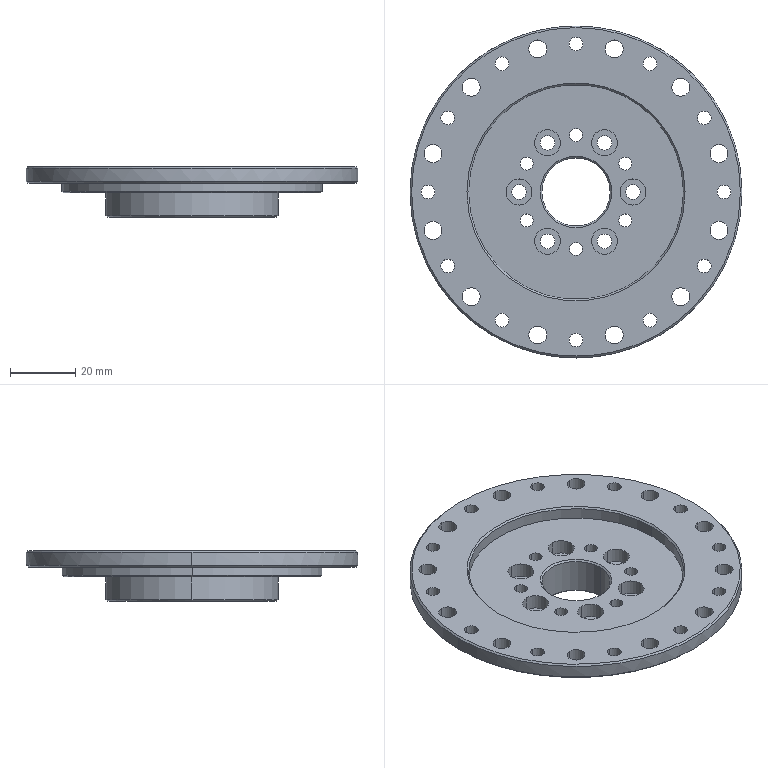NC program | NX | posted with a generic post | part box 102 x 102 x 15.5 mm
Whole program:
N10 G17 G21 G94 G90
(FLOOR_WALL_COPY_COPY , TOOL : D80)
N12 T19 M6
N14 G54
N16 G17 G0 G90 X-81.531 Y50.698 S6500 M3
N18 G43 Z30. H19
N20 Z12.
N22 G94 G1 Z9. F1500.
N24 X-75.579
N26 X75.578
N28 G2 X77.47 Y47.754 R90.667
N30 X89.618 Y15.852 R90.478
N32 G1 X-89.612
N34 G3 X-88.992 Y-18.994 R90.516
N36 G1 X89.006
N38 X94.112
N40 Z12.
N42 G0 Z30.
N44 X-81.542 Y50.698
N46 Z11.
N48 G1 Z8.
N50 X-75.59
N52 X75.572
N54 X75.681 Y50.534
N56 G2 X76.632 Y49.084 R90.524
N58 X89.618 Y15.851 R90.478
N60 G1 X-89.612
N62 G3 X-88.992 Y-18.995 R90.518
N64 G1 X89.006
N66 X94.112
N68 Z11.
N70 G0 Z30.
N72 X-81.541 Y50.699
N74 Z10.
N76 G1 Z7.
N78 X-75.589
N80 X75.571
N82 X75.653 Y50.576
N84 G2 X76.743 Y48.911 R90.596
N86 X89.618 Y15.852 R90.524
N88 G1 X-89.612
N90 G3 X-89.007 Y-18.995 R90.812
N92 G1 X89.006
N94 X94.112
N96 Z10.
N98 G0 Z30.
N100 X-81.535 Y50.701
N102 Z9.
N104 G1 Z6.
N106 X-75.582
N108 X75.576
N110 G2 X78.482 Y46.074 R90.403
N112 X88.337 Y21.908 R90.596
N114 X89.622 Y15.853 R90.962
N116 G1 X-89.622
N118 G3 X-90.747 Y6.882 R90.768
N120 X-90.99 Y1.917 R90.747
N122 G1 Y-1.978
N124 G3 X-90.558 Y-9.09 R90.747
N126 X-89.008 Y-18.995 R90.681
N128 G1 X89.009
N130 X94.116
N132 Z9.
N134 G0 Z30.
N136 X-81.535 Y50.698
N138 Z8.
N140 G1 Z5.
N142 X-75.581
N144 X75.578
N146 G2 X79.118 Y44.973 R90.403
N148 X86.435 Y28.496 R90.915
N150 X89.622 Y15.851 R90.962
N152 G1 X-89.622
N154 G3 X-90.737 Y7.019 R90.768
N156 X-90.939 Y3.54 R91.005
N158 X-90.99 Y1.854 R90.681
N160 G1 Y-1.943
N162 G3 X-89.008 Y-18.995 R90.681
N164 G1 X89.009
N166 X94.116
N168 Z8.
N170 G0 Z30.
N172 X-81.531 Y50.698
N174 Z7.
N176 G1 Z4.
N178 X-75.579
N180 X75.58
N182 G2 X88.039 Y23.072 R90.662
N184 X89.621 Y15.851 R90.915
N186 G1 X-89.617
N188 G3 X-90.99 Y1.81 R91.006
N190 G1 Y-1.809
N192 G3 X-89.003 Y-18.995 R91.006
N194 G1 X89.013
N196 X94.119
N198 Z7.
N200 G0 Z30.
N202 X-81.536 Y50.698
N204 Z6.
N206 G1 Z3.
N208 X-75.58
N210 X75.58
N212 G2 X89.013 Y18.957 R90.662
N214 X89.24 Y17.856 R90.754
N216 X89.618 Y15.851 R90.976
N218 G1 X-89.627
N220 G3 X-90.987 Y1.939 R89.934
N222 G1 X-90.99 Y1.81
N224 Y-1.83
N226 G3 X-89.005 Y-18.996 R90.93
N228 G1 X89.013
N230 X94.119
N232 Z6.
N234 G0 Z30.
N236 X-81.538 Y50.698
N238 Z5.
N240 G1 Z2.
N242 X-75.584
N244 X75.579
N246 G2 X86.561 Y28.116 R90.754
N248 X89.621 Y15.851 R90.903
N250 G1 X-89.627
N252 G3 X-90.99 Y1.827 R89.934
N254 G1 Y-1.83
N256 G3 X-89.005 Y-18.996 R90.93
N258 G1 X89.006
N260 X94.112
N262 Z5.
N264 G0 Z30.
N266 X-81.538 Y50.698
N268 Z4.
N270 G1 Z1.
N272 X-75.584
N274 X75.578
N276 G2 X89.621 Y15.851 R90.903
N278 G1 X-89.627
N280 G3 X-90.737 Y7.102 R89.96
N282 X-90.99 Y2.113 R90.464
N284 G1 Y-2.053
N286 G3 X-90.158 Y-12.385 R90.464
N288 X-89.004 Y-18.996 R90.725
N290 G1 X89.006
N292 X94.112
N294 Z4.
N296 G0 Z30.
N298 X-81.531 Y50.698
N300 Z3.
N302 G1 Z0.
N304 X-75.579
N306 X75.578
N308 G2 X80.872 Y41.745 R90.903
N310 X86.703 Y27.673 R90.662
N312 X89.621 Y15.852 R90.903
N314 G1 X-89.62
N316 G3 X-90.99 Y2.113 R90.464
N318 G1 Y-2.053
N320 G3 X-90.158 Y-12.385 R90.464
N322 G1 X-89.877 Y-14.187
N324 X-89.58 Y-16.052
N326 X-88.992 Y-18.994
N328 X89.006
N330 X94.112
N332 Z3.
N334 G0 Z30.
N336 M5
(ADAPTIVE_MILLING_COPY , TOOL : D10)
N338 T15 M6
N340 G54
N342 G17 G0 G90 X-62.764 Y0.058 S9500 M3
N344 G43 Z30. H15
N346 Z-7.35
N348 G94 G1 Z-10.35 F1000.
N350 X-60.098 Y-1.276 F3000.
N352 G3 X-56.042 Y0.058 R3.036
N354 X-55.3 Y2.889 R8.931
N356 G2 X-53.7 Y12.351 R120.532
N358 X51.154 Y20.414 R55.089
N360 X54.19 Y9.748 R75.643
N362 X-28.076 Y-47.395 R55.051
N364 X-54.993 Y-2.77 R54.915
N366 X-54.268 Y4.289 R65.456
N368 X-50.178 Y20.532 R63.779
N370 X50.149 Y20.529 R54.184
N372 X53.73 Y7.129 R62.299
N374 X-53.982 Y-4.762 R-54.197
N376 X-53.432 Y4.209 R49.517
N378 X-48.471 Y22.265 R61.183
N380 X48.962 Y21.1 R53.313
N382 X53.298 Y1.989 R55.894
N384 X-52.97 Y-6.044 R53.324
N386 X-52.525 Y4.525 R48.644
N388 X-46.394 Y24.491 R58.487
N390 X47.922 Y21.292 R52.43
N392 X52.166 Y-5.57 R53.377
N394 X-51.925 Y-7.312 R52.447
N396 X-51.665 Y4.455 R47.493
N398 X-44.724 Y25.702 R56.903
N400 X50.415 Y10.755 R51.549
N402 X-50.891 Y-8.265 R-51.555
N404 X-50.674 Y5.287 R47.612
N406 X-41.893 Y28.563 R54.436
N408 X46.25 Y20.719 R50.662
N410 X-49.822 Y-9.292 R-50.685
N412 X-49.747 Y5.645 R47.504
N414 X-39.168 Y30.799 R52.922
N416 X49.765 Y2.224 R49.828
N418 X-48.692 Y-10.483 R49.809
N420 X-48.924 Y5.238 R46.288
N422 X-38.178 Y30.622 R52.019
N424 X48.88 Y2.27 R48.942
N426 X-47.661 Y-11.044 R48.925
N428 X-47.916 Y6.054 R46.24
N430 X-35.928 Y31.919 R50.618
N432 X48.014 Y1.874 R48.06
N434 X-46.558 Y-11.846 R48.042
N436 X-46.935 Y6.622 R45.601
N438 X-33.409 Y33.31 R49.357
N440 X-44.95 Y-14.314 R-47.169
N442 X-46.245 Y5.373 R43.769
N444 X-33.737 Y31.699 R48.755
N446 X-43.928 Y-14.586 R-46.285
N448 X-45.356 Y5.38 R43.426
N450 X-32.204 Y32.007 R47.686
N452 X-43.017 Y-14.491 R-45.396
N454 X-44.97 Y-3.991 R41.694
N456 G1 X-45.148 Y-0.003
N458 X-45.149 Y0.03
N460 X-45.148 Y0.066
N462 X-44.963 Y4.076
N464 X-44.95 Y4.214
N466 X-44.404 Y8.156
N468 X-44.379 Y8.292
N470 X-43.476 Y12.168
N472 X-43.439 Y12.302
N474 X-42.186 Y16.08
N476 X-42.137 Y16.208
N478 G3 X-40.156 Y20.881 R113.964
N480 G1 X-40.009 Y21.066
N482 X-39.78 Y21.393
N484 X-37.582 Y25.016
N486 X-37.507 Y25.129
N488 X-35.153 Y28.329
N490 X-35.065 Y28.437
N492 X-32.431 Y31.408
N494 X-32.334 Y31.508
N496 X-29.44 Y34.228
N498 X-29.335 Y34.318
N500 X-26.206 Y36.763
N502 X-26.092 Y36.843
N504 X-22.754 Y38.994
N506 X-22.634 Y39.063
N508 X-19.114 Y40.901
N510 X-18.988 Y40.96
N512 X-15.315 Y42.47
N514 X-15.184 Y42.517
N516 X-11.389 Y43.687
N518 X-11.255 Y43.721
N520 X-7.369 Y44.541
N522 X-7.232 Y44.564
N524 X-3.288 Y45.027
N526 X-3.15 Y45.037
N528 X0.862 Y45.141
N530 X0.939 Y45.138
N532 X4.922 Y44.878
N534 X5.059 Y44.863
N536 X8.982 Y44.244
N538 X9.118 Y44.217
N540 X12.975 Y43.242
N542 X13.108 Y43.202
N544 X16.86 Y41.881
N546 X16.989 Y41.828
N548 X20.605 Y40.171
N550 X20.729 Y40.107
N552 X24.179 Y38.127
N554 X24.296 Y38.052
N556 X27.551 Y35.766
N558 X27.661 Y35.681
N560 X30.695 Y33.107
N562 X30.796 Y33.013
N564 X33.583 Y30.174
N566 X33.675 Y30.07
N568 X36.192 Y26.989
N570 X36.275 Y26.877
N572 X38.5 Y23.58
N574 X38.572 Y23.461
N576 X40.488 Y19.975
N578 X40.549 Y19.85
N580 X42.139 Y16.204
N582 X42.188 Y16.074
N584 X43.44 Y12.298
N586 X43.477 Y12.164
N588 X44.379 Y8.29
N590 X44.405 Y8.153
N592 X44.95 Y4.213
N594 X44.963 Y4.074
N596 X45.148 Y0.066
N598 X45.149 Y0.026
N600 Y0.001
N602 G2 X43.798 Y-10.957 R48.696
N604 X38.052 Y-24.296 R47.114
N606 G1 X37.981 Y-24.407
N608 X35.656 Y-27.692
N610 X35.57 Y-27.803
N612 X32.956 Y-30.857
N614 X32.859 Y-30.96
N616 X29.975 Y-33.76
N618 X29.87 Y-33.853
N620 X26.74 Y-36.376
N622 X26.627 Y-36.459
N624 X23.278 Y-38.683
N626 X23.157 Y-38.755
N628 X19.618 Y-40.662
N630 X19.491 Y-40.723
N632 X15.791 Y-42.295
N634 X15.66 Y-42.344
N636 X11.831 Y-43.569
N638 X11.695 Y-43.606
N640 X7.77 Y-44.473
N642 X7.631 Y-44.497
N644 X3.643 Y-45.
N646 X3.503 Y-45.011
N648 X-0.566 Y-45.145
N650 X-0.63 Y-45.144
N652 X-4.669 Y-44.905
N654 X-4.808 Y-44.89
N656 X-8.783 Y-44.284
N658 X-8.92 Y-44.257
N660 X-12.822 Y-43.288
N662 X-12.957 Y-43.248
N664 X-16.752 Y-41.924
N666 X-16.883 Y-41.871
N668 X-20.541 Y-40.203
N670 X-20.666 Y-40.139
N672 X-24.154 Y-38.142
N674 X-24.273 Y-38.066
N676 X-27.563 Y-35.756
N678 X-27.674 Y-35.67
N680 X-30.738 Y-33.067
N682 X-30.84 Y-32.971
N684 X-33.651 Y-30.097
N686 X-33.745 Y-29.992
N688 X-36.279 Y-26.872
N690 X-36.362 Y-26.759
N692 X-38.599 Y-23.417
N694 X-38.671 Y-23.298
N696 X-40.562 Y-19.823
N698 X-40.623 Y-19.698
N700 X-42.192 Y-16.065
N702 X-42.241 Y-15.936
N704 X-43.474 Y-12.176
N706 X-43.511 Y-12.043
N708 X-44.399 Y-8.186
N710 X-44.423 Y-8.05
N712 X-44.936 Y-4.285
N714 G3 X-45.605 Y-2.762 R3.1
N716 G1 X-51.263 Y4.072
N718 Z-7.35
N720 G0 Z30.
N722 X-50.739 Y-0.03
N724 Z-4.527
N726 G1 Z-7.527 F1000.
N728 G3 X-44.739 Y-0.03 R3.008 F3000.
N730 G1 X-44.738 Y0.003
N732 X-44.562 Y3.949
N734 X-44.549 Y4.087
N736 X-44.021 Y7.966
N738 X-43.997 Y8.102
N740 X-43.12 Y11.918
N742 X-43.083 Y12.051
N744 X-41.864 Y15.772
N746 X-41.815 Y15.901
N748 X-40.265 Y19.496
N750 X-40.204 Y19.62
N752 X-38.335 Y23.06
N754 X-38.264 Y23.178
N756 X-36.09 Y26.435
N758 X-36.009 Y26.546
N760 X-33.55 Y29.593
N762 X-33.458 Y29.697
N764 X-30.734 Y32.508
N766 X-30.633 Y32.603
N768 X-27.665 Y35.156
N770 X-27.557 Y35.242
N772 X-24.37 Y37.516
N774 X-24.254 Y37.591
N776 X-20.874 Y39.568
N778 X-20.752 Y39.632
N780 X-17.207 Y41.295
N782 X-17.08 Y41.348
N784 X-13.399 Y42.683
N786 X-13.267 Y42.724
N788 X-9.481 Y43.72
N790 X-9.346 Y43.749
N792 X-5.485 Y44.399
N794 X-5.348 Y44.416
N796 X-1.433 Y44.714
N798 X-1.333 Y44.718
N800 X2.609 Y44.66
N802 X2.747 Y44.652
N804 X6.641 Y44.241
N806 X6.776 Y44.22
N808 G2 X14.482 Y42.328 R51.813
N810 X21.733 Y39.103 R51.819
N812 X28.3 Y34.648 R51.819
N814 X33.977 Y29.102 R51.819
N816 X38.584 Y22.641 R51.819
N818 X41.977 Y15.468 R51.819
N820 X44.05 Y7.807 R51.819
N822 X44.738 Y-0.067 R52.052
N824 G1 X44.542 Y-4.165
N826 X44.528 Y-4.308
N828 X43.953 Y-8.334
N830 X43.926 Y-8.475
N832 X42.975 Y-12.429
N834 X42.935 Y-12.567
N836 X41.616 Y-16.414
N838 X41.563 Y-16.547
N840 X39.889 Y-20.254
N842 X39.824 Y-20.381
N844 X37.808 Y-23.914
N846 X37.732 Y-24.034
N848 X35.447 Y-27.292
N850 X35.361 Y-27.403
N852 X32.786 Y-30.437
N854 X32.69 Y-30.54
N856 X29.847 Y-33.324
N858 X29.742 Y-33.417
N860 X26.655 Y-35.928
N862 X26.542 Y-36.012
N864 X23.237 Y-38.228
N866 X23.117 Y-38.301
N868 X19.622 Y-40.203
N870 X19.496 Y-40.265
N872 X15.84 Y-41.838
N874 X15.709 Y-41.887
N876 X11.924 Y-43.118
N878 X11.789 Y-43.155
N880 X7.907 Y-44.032
N882 X7.769 Y-44.056
N884 X3.823 Y-44.573
N886 X3.683 Y-44.584
N888 X-0.351 Y-44.737
N890 X-0.405 Y-44.736
N892 X-4.407 Y-44.519
N894 X-4.547 Y-44.505
N896 X-8.484 Y-43.924
N898 X-8.622 Y-43.898
N900 X-12.489 Y-42.958
N902 X-12.623 Y-42.918
N904 X-16.387 Y-41.627
N906 X-16.518 Y-41.575
N908 X-20.147 Y-39.943
N910 X-20.272 Y-39.879
N912 X-23.736 Y-37.92
N914 X-23.855 Y-37.845
N916 X-27.124 Y-35.576
N918 X-27.235 Y-35.49
N920 X-30.281 Y-32.93
N922 X-30.385 Y-32.834
N924 X-33.182 Y-30.004
N926 X-33.276 Y-29.9
N928 X-35.802 Y-26.825
N930 X-35.886 Y-26.712
N932 X-38.118 Y-23.417
N934 X-38.191 Y-23.298
N936 X-40.097 Y-19.839
N938 X-40.159 Y-19.714
N940 X-41.741 Y-16.094
N942 X-41.791 Y-15.964
N944 X-43.036 Y-12.216
N946 X-43.074 Y-12.082
N948 X-43.972 Y-8.235
N950 X-43.997 Y-8.098
N952 X-44.54 Y-4.185
N954 X-44.553 Y-4.047
N956 X-44.738 Y-0.066
N958 X-44.739 Y-0.03
N960 G3 X-49.093 Y2.625 R3.033
N962 G1 X-51.065 Y1.666
N964 Z-4.527
N966 G0 Z30.
N968 X-51.461 Y-0.007
N970 Z-4.35
N972 G1 Z-7.35 F1000.
N974 X-48.795 Y-1.342 F3000.
N976 G3 X-44.739 Y-0.007 R3.036
N978 X-44.026 Y2.524 R8.51
N980 G2 X-42.34 Y11.156 R94.212
N982 X-24.606 Y-36.198 R-43.767
N984 X-35.17 Y-25.945 R40.986
N986 X-39.985 Y-17.772 R52.804
N988 X-43.642 Y-2.7 R41.174
N990 X-42.746 Y5.142 R57.43
N992 X-36.161 Y23.032 R46.618
N994 X-32.554 Y-27.868 R-42.869
N996 X-40.322 Y-14.541 R46.038
N998 X-42.636 Y-3.727 R37.084
N1000 X-41.47 Y7.29 R50.549
N1002 X-28.657 Y30.669 R43.444
N1004 X-31.592 Y-27.599 R-41.971
N1006 X-41.278 Y-7.582 R42.621
N1008 X-41.33 Y2.777 R34.387
N1010 X-35.067 Y21.401 R46.274
N1012 X-29.724 Y-28.323 R-41.072
N1014 X-40.27 Y-7.999 R41.445
N1016 X-40.253 Y4.146 R37.044
N1018 X-32.303 Y23.888 R43.662
N1020 X-37.007 Y-15.587 R-40.169
N1022 X-39.555 Y2.609 R34.322
N1024 X-31.205 Y23.847 R42.831
N1026 X-27.853 Y-27.651 R-39.266
N1028 X-38.227 Y-8.799 R39.001
N1030 X-38.127 Y6.003 R37.563
N1032 X-25.207 Y28.916 R40.16
N1034 X-27.638 Y-26.564 R-38.358
N1036 X-37.324 Y-8.565 R37.548
N1038 X-36.801 Y7.894 R37.935
N1040 X-19.615 Y31.904 R38.648
N1042 X-35.356 Y-12.27 R-37.447
N1044 X-36.552 Y4.614 R34.662
N1046 X-23.298 Y28.148 R38.436
N1048 X-33.855 Y-13.677 R-36.535
N1050 X-35.549 Y5.096 R33.978
N1052 X-21.388 Y28.488 R37.269
N1054 X-32.112 Y-15.358 R-35.619
N1056 X-34.704 Y4.648 R33.081
N1058 X-19.952 Y28.394 R36.267
N1060 X-30.514 Y-16.47 R-34.699
N1062 X-33.719 Y4.965 R32.425
N1064 X-17.409 Y28.949 R35.146
N1066 X-28.732 Y-17.71 R-33.776
N1068 X-32.704 Y5.381 R31.726
N1070 X-14.854 Y29.301 R33.998
N1072 X-28.114 Y-16.935 R-32.847
N1074 X-31.774 Y5.335 R31.023
N1076 X-13.556 Y28.897 R33.011
N1078 X-26.732 Y-17.386 R-31.914
N1080 X-31.368 Y-4.006 R29.457
N1082 X-31.648 Y0.073 R38.073
N1084 X-30.896 Y6.847 R36.815
N1086 X-28.73 Y13.267 R36.514
N1088 X-25.247 Y19.08 R36.514
N1090 X-20.607 Y24.017 R36.514
N1092 X-15.021 Y27.853 R36.514
N1094 X-8.747 Y30.413 R36.514
N1096 X-2.072 Y31.578 R36.514
N1098 X4.535 Y31.319 R36.568
N1100 X11.385 Y29.526 R36.166
N1102 G1 X14.395 Y28.182
N1104 X14.544 Y28.106
N1106 X17.389 Y26.44
N1108 X17.528 Y26.348
N1110 X20.174 Y24.382
N1112 X20.302 Y24.275
N1114 X22.717 Y22.031
N1116 X22.833 Y21.911
N1118 X24.989 Y19.417
N1120 X25.091 Y19.285
N1122 X26.961 Y16.57
N1124 X27.048 Y16.428
N1126 X28.61 Y13.524
N1128 X28.681 Y13.374
N1130 X29.916 Y10.317
N1132 X29.97 Y10.159
N1134 X30.865 Y6.986
N1136 X30.901 Y6.824
N1138 X31.443 Y3.572
N1140 X31.462 Y3.406
N1142 X31.648 Y0.073
N1144 X31.649 Y0.025
N1146 X31.648 Y-0.005
N1148 G2 X29.327 Y-11.893 R33.08
N1150 X26.394 Y-17.459 R35.835
N1152 G1 X24.383 Y-20.171
N1154 X24.274 Y-20.302
N1156 X21.977 Y-22.769
N1158 X21.854 Y-22.887
N1160 X19.296 Y-25.081
N1162 X19.161 Y-25.185
N1164 X16.374 Y-27.08
N1166 X16.228 Y-27.168
N1168 X13.246 Y-28.74
N1170 X13.091 Y-28.811
N1172 X9.953 Y-30.039
N1174 X9.791 Y-30.093
N1176 X6.535 Y-30.963
N1178 X6.368 Y-30.998
N1180 X3.035 Y-31.499
N1182 X2.865 Y-31.515
N1184 X-0.559 Y-31.643
N1186 X-0.645 Y-31.64
N1188 X-4.034 Y-31.387
N1190 X-4.203 Y-31.365
N1192 X-7.515 Y-30.74
N1194 X-7.68 Y-30.699
N1196 X-10.902 Y-29.708
N1198 X-11.062 Y-29.649
N1200 X-14.152 Y-28.304
N1202 X-14.304 Y-28.228
N1204 X-17.225 Y-26.546
N1206 X-17.368 Y-26.453
N1208 X-20.083 Y-24.456
N1210 X-20.214 Y-24.348
N1212 X-22.689 Y-22.06
N1214 X-22.808 Y-21.937
N1216 X-25.011 Y-19.387
N1218 X-25.116 Y-19.252
N1220 X-27.021 Y-16.471
N1222 X-27.109 Y-16.327
N1224 X-28.655 Y-13.428
N1226 X-28.725 Y-13.278
N1228 X-29.947 Y-10.227
N1230 X-30.001 Y-10.07
N1232 X-30.883 Y-6.904
N1234 X-30.919 Y-6.742
N1236 X-31.373 Y-3.979
N1238 G3 X-32.201 Y-2.346 R3.075
N1240 G1 X-37.769 Y3.321
N1242 Z-4.35
N1244 G0 Z30.
N1246 M5
(FLOOR_WALL_COPY_1_COPY_COPY , TOOL : D10JING)
N1248 T14 M6
N1250 G54
N1252 G17 G0 G90 X-0.262 Y-47.996 S9500 M3
N1254 G43 Z30. H14
N1256 Z-4.5
N1258 G94 G1 Z-7.5 F1000.
N1260 X0. Y-41.001
N1262 G2 X38.166 Y14.979 R-41.001 F1200.
N1264 X-4.986 Y-40.67 R40.973
N1266 X-7.12 Y-38.046 R2.441
N1268 G1 X-7.073 Y-37.474
N1270 G3 X-8.944 Y-34.848 R2.5
N1272 G2 X-28.144 Y22.444 R35.974
N1274 X34.398 Y10.61 R35.997
N1276 X-1.265 Y-35.954 R35.972
N1278 X-3.149 Y-34.99 R2.5
N1280 G1 X-5.331 Y-32.184
N1282 G3 X-6.776 Y-31.274 R2.5
N1284 G2 X-3.937 Y-31.757 R-32.
N1286 G1 X-4.306 Y-34.734
N1288 X-3.875 Y-31.261 F1000.
N1290 G2 X-31.261 Y3.875 R31.5 F1200.
N1292 X-3.875 Y-31.261 R-31.5
N1294 G1 X-4.306 Y-34.734
N1296 Z-4.5
N1298 G0 Z30.
N1300 X-0.239 Y-58.997
N1302 Z-7.5
N1304 G1 Z-10.5 F1000.
N1306 X0. Y-52.001
N1308 G2 X46.171 Y23.924 R-52.001 F1200.
N1310 X-4.99 Y-51.731 R51.972
N1312 X-7.177 Y-49.116 R2.43
N1314 G1 X-7.146 Y-48.728
N1316 G3 X-9.151 Y-46.074 R2.5
N1318 G2 X-36.457 Y29.66 R46.973
N1320 X44.284 Y15.739 R46.998
N1322 X-3.299 Y-46.856 R46.969
N1324 X-4.028 Y-46.48 R1.041
N1326 G1 X-4.653 Y-45.723
N1328 G3 X-5.711 Y-45.14 R1.638
N1330 G2 X-4.339 Y-45.293 R-45.5
N1332 G1 X-4.625 Y-48.279
N1334 X-4.291 Y-44.795 F1000.
N1336 G2 X-44.795 Y4.291 R45. F1200.
N1338 X-4.291 Y-44.795 R-45.
N1340 G1 X-4.625 Y-48.279
N1342 Z-7.5
N1344 G0 Z30.
N1346 M5
(PLANAR_MILL_COPY_COPY_COPY_COPY_COPY_COPY_1_COPY_1 , TOOL : D6A45)
N1348 T01 M6
N1350 G54
N1352 G17 G0 G90 X9.1 Y-0.866 S9500 M3
N1354 G43 Z30. H1
N1356 Z0.3
N1358 G94 G1 Z-1.2 F1250.
N1360 G3 X9.6 Y0. R1.
N1362 X0. Y9.6 R9.6
N1364 X9.6 Y0. R-9.6
N1366 X9.1 Y0.866 R1.
N1368 G1 Z0.3
N1370 G0 Z30.
N1372 X27.7
N1374 Z0.3
N1376 G1 Z-1.2
N1378 G3 X27.2 Y0. R1.
N1380 G2 X0. Y-27.2 R27.2
N1382 X27.2 Y0. R-27.2
N1384 G3 X27.7 Y-0.866 R1.
N1386 G1 Z0.3
N1388 G0 Z30.
(PLANAR_MILL_COPY_COPY_COPY_COPY_COPY_COPY_1_COPY_1_COPY , TOOL : D6A45)
N1390 X-41.2
N1392 Z-7.2
N1394 G1 Z-8.7
N1396 G3 X-40.7 Y0. R1.
N1398 G2 X0. Y40.7 R40.7
N1400 X-40.7 Y0. R-40.7
N1402 G3 X-41.2 Y0.866 R1.
N1404 G1 Z-7.2
N1406 G0 Z30.
(PLANAR_MILL_COPY_COPY_COPY_COPY_COPY_COPY_1_COPY_1_COPY_COPY , TOOL : D6A45)
N1408 X-52.2 Y-0.866
N1410 Z-10.2
N1412 G1 Z-11.7
N1414 G3 X-51.7 Y0. R1.
N1416 G2 X0. Y51.7 R51.7
N1418 X-51.7 Y0. R-51.7
N1420 G3 X-52.2 Y0.866 R1.
N1422 G1 Z-10.2
N1424 G0 Z30.
N1426 M5
N1428 M2